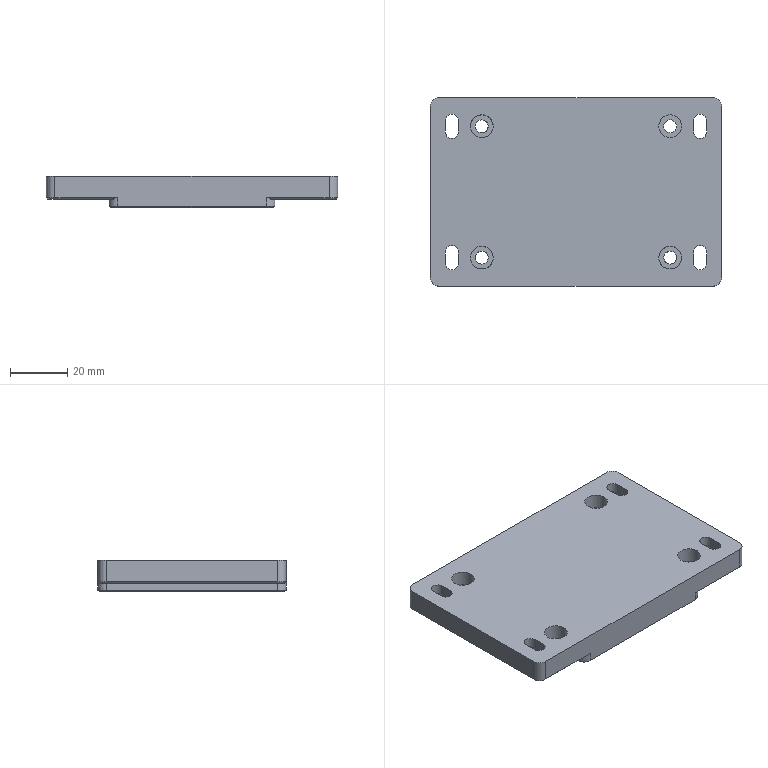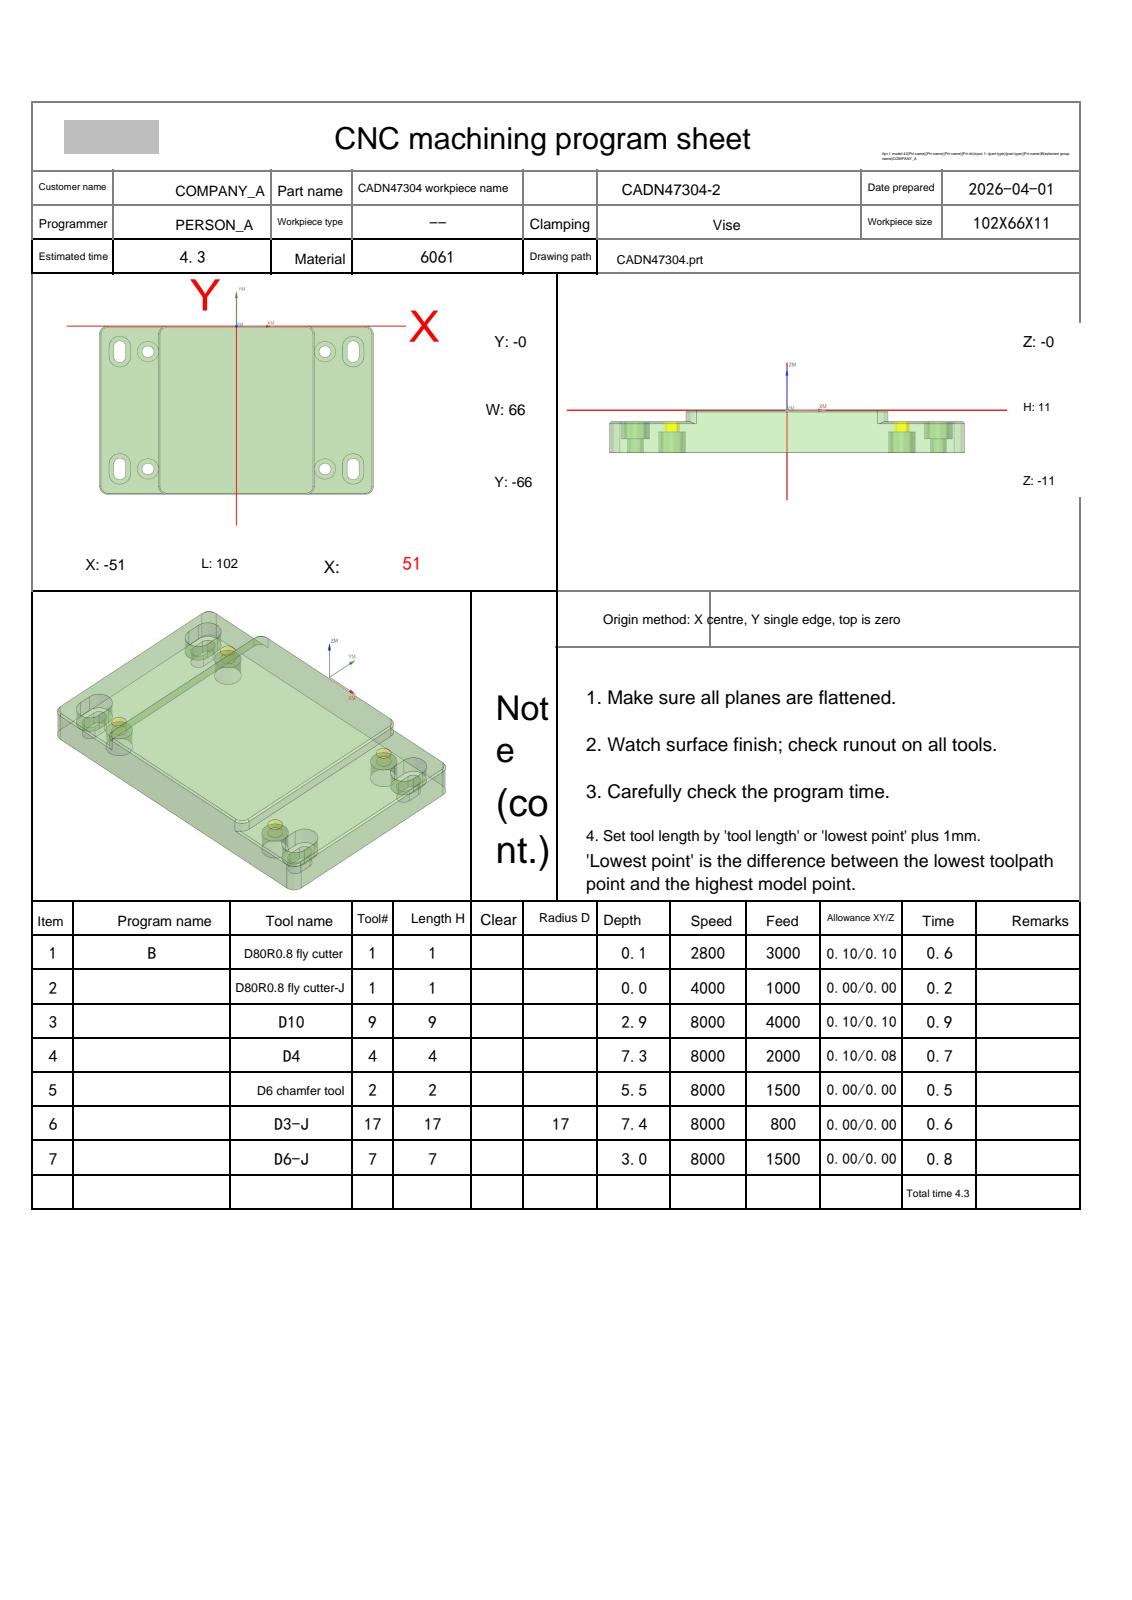NC program | NX | posted by the shop | part box 102 x 66 x 11 mm
Whole program:
%
O0001
(Machine time: 5.73 MIN)
(===Total Tool:6===)
(T1=D80R0.8 fly cutter D=80.  R=0.8  D-  H01 Z=-0.   )
(T9=D10     D=10.  R=0.   D-  H09 Z=-2.9  )
(T4=D4      D=4.   R=0.   D-  H04 Z=-7.34 )
(T2=D6 chamfer tool   D=6.   R=0.   D-  H02 Z=-5.55 )
(T17=D3-J   D=3.   R=0.   D17 H17 Z=-7.4  )
(T7=D6-J    D=6.   R=0.   D7  H07 Z=-3.   )
G80 G90 G17 G49 G40
G91 G28 Z0
M01
N1 T01 M06
(D80R0.8 fly cutter  D=80. R=0.8 H=01 ce=0.10 di=0.10)
G00 G90 G54 X103.097 Y-32.998 M03 S2800
G43 H01 Z20.
M08
Z5.014
G01 Z3.014 F3000.
X91.097
X-91.097 Y-33.002
X-103.097
Z5.014
G00 X103.097 Y-32.998
Z4.529
G01 Z2.529
X91.097
X-91.097 Y-33.002
X-103.097
Z4.529
G00 X103.097 Y-32.998
Z4.043
G01 Z2.043
X91.097
X-91.097 Y-33.002
X-103.097
Z4.043
G00 X103.097 Y-32.998
Z3.557
G01 Z1.557
X91.097
X-91.097 Y-33.002
X-103.097
Z3.557
G00 Z20.
X103.097 Y-32.998
Z3.071
G01 Z1.071
X91.097
X-91.097 Y-33.002
X-103.097
Z3.071
G00 Z20.
X103.097 Y-32.998
Z2.586
G01 Z.586
X91.097
X-91.097 Y-33.002
X-103.097
Z2.586
G00 Z20.
X103.097 Y-32.998
Z2.1
G01 Z.1
X91.097
X-91.097 Y-33.002
X-103.097
Z2.1
G00 Z20.
G91 G28 Z0.0
M05
M09
G91 G28 Z0.0
M01
N2 T01 M06
(D80R0.8 fly cutter-J  D=80. R=0.8 H=01 ce=0.00 di=0.00)
G00 G90 G54 X102.999 Y-32.998 M03 S4000
G43 H01 Z20.
M08
Z2.
G01 Z0.0 F1000.
X90.999
X-90.999 Y-33.002
X-102.999
Z2.
G00 Z20.
G91 G28 Z0.0
M05
M09
G91 G28 Z0.0
M01
N3 T09 M06
(D10  D=10. R=0. H=09 ce=0.10 di=0.10)
G00 G90 G54 X-52.925 Y6.273 M03 S8000
G43 H09 Z13.5
M08
Z.92
G01 Z-.58 F4000.
X-53.701 Y1.718
G03 X-54.1 Y-3. I27.701 J-4.718
G01 Y-63.
G03 X-53.748 Y-67.436 I28.1 J0.0
X-53.504 Y-67.946 I.987 J.158
X-48.778 Y-70.359 I5.504 J4.946
G01 X-48.715 Y-70.362
G03 X-48.115 Y-69.762 I0.0 J.6
G01 X-48.14 Y-69.591
G02 X-49.1 Y-63. I22.14 J6.591
G01 Y-3.
G02 X-48.11 Y3.69 I23.1 J0.0
X-47.153 Y4.4 I.957 J-.29
G01 X-40.704
G02 X-40.104 Y3.8 I0.0 J-.6
X-40.159 Y3.548 I-.6 J0.0
G03 X-41.6 Y-3. I14.159 J-6.548
G01 Y-63.
G03 X-39.963 Y-69.956 I15.6 J0.0
X-39.258 Y-70.492 I.895 J.446
G01 X-29.89 Y-72.296
X-29.701 Y-72.314
G03 X-28.701 Y-71.314 I0.0 J1.
X-29.294 Y-70.4 I-1. J0.0
G02 X-34.1 Y-63. I3.294 J7.4
G01 Y-3.
G02 X-29.294 Y4.4 I8.1 J0.0
G01 X-20.982 Y8.1
Z.92
G00 X-52.925 Y6.273
Z.34
G01 Z-1.16
X-53.701 Y1.718
G03 X-54.1 Y-3. I27.701 J-4.718
G01 Y-63.
G03 X-53.748 Y-67.436 I28.1 J0.0
X-53.504 Y-67.946 I.987 J.158
X-48.778 Y-70.359 I5.504 J4.946
G01 X-48.715 Y-70.362
G03 X-48.115 Y-69.762 I0.0 J.6
G01 X-48.14 Y-69.591
G02 X-49.1 Y-63. I22.14 J6.591
G01 Y-3.
G02 X-48.11 Y3.69 I23.1 J0.0
X-47.153 Y4.4 I.957 J-.29
G01 X-40.704
G02 X-40.104 Y3.8 I0.0 J-.6
X-40.159 Y3.548 I-.6 J0.0
G03 X-41.6 Y-3. I14.159 J-6.548
G01 Y-63.
G03 X-39.963 Y-69.956 I15.6 J0.0
X-39.258 Y-70.492 I.895 J.446
G01 X-29.89 Y-72.296
X-29.701 Y-72.314
G03 X-28.701 Y-71.314 I0.0 J1.
X-29.294 Y-70.4 I-1. J0.0
G02 X-34.1 Y-63. I3.294 J7.4
G01 Y-3.
G02 X-29.294 Y4.4 I8.1 J0.0
G01 X-20.982 Y8.1
Z.34
G00 X-52.925 Y6.273
Z-.24
G01 Z-1.74
X-53.701 Y1.718
G03 X-54.1 Y-3. I27.701 J-4.718
G01 Y-63.
G03 X-53.748 Y-67.436 I28.1 J0.0
X-53.504 Y-67.946 I.987 J.158
X-48.778 Y-70.359 I5.504 J4.946
G01 X-48.715 Y-70.362
G03 X-48.115 Y-69.762 I0.0 J.6
G01 X-48.14 Y-69.591
G02 X-49.1 Y-63. I22.14 J6.591
G01 Y-3.
G02 X-48.11 Y3.69 I23.1 J0.0
X-47.153 Y4.4 I.957 J-.29
G01 X-40.704
G02 X-40.104 Y3.8 I0.0 J-.6
X-40.159 Y3.548 I-.6 J0.0
G03 X-41.6 Y-3. I14.159 J-6.548
G01 Y-63.
G03 X-39.963 Y-69.956 I15.6 J0.0
X-39.258 Y-70.492 I.895 J.446
G01 X-29.89 Y-72.296
X-29.701 Y-72.314
G03 X-28.701 Y-71.314 I0.0 J1.
X-29.294 Y-70.4 I-1. J0.0
G02 X-34.1 Y-63. I3.294 J7.4
G01 Y-3.
G02 X-29.294 Y4.4 I8.1 J0.0
G01 X-20.982 Y8.1
Z-.24
G00 X-52.925 Y6.273
Z-.82
G01 Z-2.32
X-53.701 Y1.718
G03 X-54.1 Y-3. I27.701 J-4.718
G01 Y-63.
G03 X-53.748 Y-67.436 I28.1 J0.0
X-53.504 Y-67.946 I.987 J.158
X-48.778 Y-70.359 I5.504 J4.946
G01 X-48.715 Y-70.362
G03 X-48.115 Y-69.762 I0.0 J.6
G01 X-48.14 Y-69.591
G02 X-49.1 Y-63. I22.14 J6.591
G01 Y-3.
G02 X-48.11 Y3.69 I23.1 J0.0
X-47.153 Y4.4 I.957 J-.29
G01 X-40.704
G02 X-40.104 Y3.8 I0.0 J-.6
X-40.159 Y3.548 I-.6 J0.0
G03 X-41.6 Y-3. I14.159 J-6.548
G01 Y-63.
G03 X-39.963 Y-69.956 I15.6 J0.0
X-39.258 Y-70.492 I.895 J.446
G01 X-29.89 Y-72.296
X-29.701 Y-72.314
G03 X-28.701 Y-71.314 I0.0 J1.
X-29.294 Y-70.4 I-1. J0.0
G02 X-34.1 Y-63. I3.294 J7.4
G01 Y-3.
G02 X-29.294 Y4.4 I8.1 J0.0
G01 X-20.982 Y8.1
Z-.82
G00 X-52.925 Y6.273
Z-1.4
G01 Z-2.9
X-53.701 Y1.718
G03 X-54.1 Y-3. I27.701 J-4.718
G01 Y-63.
G03 X-53.748 Y-67.436 I28.1 J0.0
X-53.504 Y-67.946 I.987 J.158
X-48.778 Y-70.359 I5.504 J4.946
G01 X-48.715 Y-70.362
G03 X-48.115 Y-69.762 I0.0 J.6
G01 X-48.14 Y-69.591
G02 X-49.1 Y-63. I22.14 J6.591
G01 Y-3.
G02 X-48.11 Y3.69 I23.1 J0.0
X-47.153 Y4.4 I.957 J-.29
G01 X-40.704
G02 X-40.104 Y3.8 I0.0 J-.6
X-40.159 Y3.548 I-.6 J0.0
G03 X-41.6 Y-3. I14.159 J-6.548
G01 Y-63.
G03 X-39.963 Y-69.956 I15.6 J0.0
X-39.258 Y-70.492 I.895 J.446
G01 X-29.89 Y-72.296
X-29.701 Y-72.314
G03 X-28.701 Y-71.314 I0.0 J1.
X-29.294 Y-70.4 I-1. J0.0
G02 X-34.1 Y-63. I3.294 J7.4
G01 Y-3.
G02 X-29.294 Y4.4 I8.1 J0.0
G01 X-20.982 Y8.1
Z-1.4
G00 Z13.5
X52.925 Y-72.273
Z.92
G01 Z-.58
X53.701 Y-67.718
G03 X54.1 Y-63. I-27.701 J4.718
G01 Y-3.
G03 X53.748 Y1.436 I-28.1 J0.0
X53.504 Y1.946 I-.987 J-.158
X48.778 Y4.359 I-5.504 J-4.946
G01 X48.715 Y4.362
G03 X48.115 Y3.762 I0.0 J-.6
G01 X48.14 Y3.591
G02 X49.1 Y-3. I-22.14 J-6.591
G01 Y-63.
G02 X48.11 Y-69.69 I-23.1 J0.0
X47.153 Y-70.4 I-.957 J.29
G01 X40.704
G02 X40.104 Y-69.8 I0.0 J.6
X40.159 Y-69.548 I.6 J0.0
G03 X41.6 Y-63. I-14.159 J6.548
G01 Y-3.
G03 X39.963 Y3.956 I-15.6 J0.0
X39.258 Y4.492 I-.895 J-.446
G01 X29.89 Y6.296
X29.701 Y6.314
G03 X28.701 Y5.314 I0.0 J-1.
X29.294 Y4.4 I1. J0.0
G02 X34.1 Y-3. I-3.294 J-7.4
G01 Y-63.
G02 X29.294 Y-70.4 I-8.1 J0.0
G01 X20.982 Y-74.1
Z.92
G00 X52.925 Y-72.273
Z.34
G01 Z-1.16
X53.701 Y-67.718
G03 X54.1 Y-63. I-27.701 J4.718
G01 Y-3.
G03 X53.748 Y1.436 I-28.1 J0.0
X53.504 Y1.946 I-.987 J-.158
X48.778 Y4.359 I-5.504 J-4.946
G01 X48.715 Y4.362
G03 X48.115 Y3.762 I0.0 J-.6
G01 X48.14 Y3.591
G02 X49.1 Y-3. I-22.14 J-6.591
G01 Y-63.
G02 X48.11 Y-69.69 I-23.1 J0.0
X47.153 Y-70.4 I-.957 J.29
G01 X40.704
G02 X40.104 Y-69.8 I0.0 J.6
X40.159 Y-69.548 I.6 J0.0
G03 X41.6 Y-63. I-14.159 J6.548
G01 Y-3.
G03 X39.963 Y3.956 I-15.6 J0.0
X39.258 Y4.492 I-.895 J-.446
G01 X29.89 Y6.296
X29.701 Y6.314
G03 X28.701 Y5.314 I0.0 J-1.
X29.294 Y4.4 I1. J0.0
G02 X34.1 Y-3. I-3.294 J-7.4
G01 Y-63.
G02 X29.294 Y-70.4 I-8.1 J0.0
G01 X20.982 Y-74.1
Z.34
G00 X52.925 Y-72.273
Z-.24
G01 Z-1.74
X53.701 Y-67.718
G03 X54.1 Y-63. I-27.701 J4.718
G01 Y-3.
G03 X53.748 Y1.436 I-28.1 J0.0
X53.504 Y1.946 I-.987 J-.158
X48.778 Y4.359 I-5.504 J-4.946
G01 X48.715 Y4.362
G03 X48.115 Y3.762 I0.0 J-.6
G01 X48.14 Y3.591
G02 X49.1 Y-3. I-22.14 J-6.591
G01 Y-63.
G02 X48.11 Y-69.69 I-23.1 J0.0
X47.153 Y-70.4 I-.957 J.29
G01 X40.704
G02 X40.104 Y-69.8 I0.0 J.6
X40.159 Y-69.548 I.6 J0.0
G03 X41.6 Y-63. I-14.159 J6.548
G01 Y-3.
G03 X39.963 Y3.956 I-15.6 J0.0
X39.258 Y4.492 I-.895 J-.446
G01 X29.89 Y6.296
X29.701 Y6.314
G03 X28.701 Y5.314 I0.0 J-1.
X29.294 Y4.4 I1. J0.0
G02 X34.1 Y-3. I-3.294 J-7.4
G01 Y-63.
G02 X29.294 Y-70.4 I-8.1 J0.0
G01 X20.982 Y-74.1
Z-.24
G00 X52.925 Y-72.273
Z-.82
G01 Z-2.32
X53.701 Y-67.718
G03 X54.1 Y-63. I-27.701 J4.718
G01 Y-3.
G03 X53.748 Y1.436 I-28.1 J0.0
X53.504 Y1.946 I-.987 J-.158
X48.778 Y4.359 I-5.504 J-4.946
G01 X48.715 Y4.362
G03 X48.115 Y3.762 I0.0 J-.6
G01 X48.14 Y3.591
G02 X49.1 Y-3. I-22.14 J-6.591
G01 Y-63.
G02 X48.11 Y-69.69 I-23.1 J0.0
X47.153 Y-70.4 I-.957 J.29
G01 X40.704
G02 X40.104 Y-69.8 I0.0 J.6
X40.159 Y-69.548 I.6 J0.0
G03 X41.6 Y-63. I-14.159 J6.548
G01 Y-3.
G03 X39.963 Y3.956 I-15.6 J0.0
X39.258 Y4.492 I-.895 J-.446
G01 X29.89 Y6.296
X29.701 Y6.314
G03 X28.701 Y5.314 I0.0 J-1.
X29.294 Y4.4 I1. J0.0
G02 X34.1 Y-3. I-3.294 J-7.4
G01 Y-63.
G02 X29.294 Y-70.4 I-8.1 J0.0
G01 X20.982 Y-74.1
Z-.82
G00 X52.925 Y-72.273
Z-1.4
G01 Z-2.9
X53.701 Y-67.718
G03 X54.1 Y-63. I-27.701 J4.718
G01 Y-3.
G03 X53.748 Y1.436 I-28.1 J0.0
X53.504 Y1.946 I-.987 J-.158
X48.778 Y4.359 I-5.504 J-4.946
G01 X48.715 Y4.362
G03 X48.115 Y3.762 I0.0 J-.6
G01 X48.14 Y3.591
G02 X49.1 Y-3. I-22.14 J-6.591
G01 Y-63.
G02 X48.11 Y-69.69 I-23.1 J0.0
X47.153 Y-70.4 I-.957 J.29
G01 X40.704
G02 X40.104 Y-69.8 I0.0 J.6
X40.159 Y-69.548 I.6 J0.0
G03 X41.6 Y-63. I-14.159 J6.548
G01 Y-3.
G03 X39.963 Y3.956 I-15.6 J0.0
X39.258 Y4.492 I-.895 J-.446
G01 X29.89 Y6.296
X29.701 Y6.314
G03 X28.701 Y5.314 I0.0 J-1.
X29.294 Y4.4 I1. J0.0
G02 X34.1 Y-3. I-3.294 J-7.4
G01 Y-63.
G02 X29.294 Y-70.4 I-8.1 J0.0
G01 X20.982 Y-74.1
Z-1.4
G00 Z13.5
G91 G28 Z0.0
M05
M09
G91 G28 Z0.0
M01
N4 T04 M06
(D4  D=4. R=0. H=04 ce=0.10 di=0.08)
G00 G90 G54 X-45.233 Y-12.757 M03 S8000
G43 H04 Z20.
M08
Z-2.2
G01 X-45.112 Y-13.062 Z-2.217 F2000.
X-44.562 Y-13.612 Z-2.258
X-43.839 Y-13.9 Z-2.299
X-43.161 Z-2.334
X-42.438 Y-13.612 Z-2.375
X-41.888 Y-13.062 Z-2.416
X-41.6 Y-12.339 Z-2.457
Y-7.661 Z-2.702
X-41.839 Y-7.017 Z-2.738
X-42.282 Y-6.503 Z-2.773
X-42.696 Y-6.246 Z-2.799
X-43.161 Y-6.1 Z-2.824
X-43.839 Z-2.86
X-44.562 Y-6.388 Z-2.901
X-45.112 Y-6.938 Z-2.941
X-45.4 Y-7.661 Z-2.982
Y-8. Z-3.
Y-12. Z-3.058
G03 X-43.5 Y-13.9 Z-3.101 I1.9 J0.0
X-41.6 Y-12. Z-3.145 I0.0 J1.9
G01 Y-8. Z-3.203
G03 X-42.061 Y-6.76 Z-3.222 I-1.9 J0.0
X-43.5 Y-6.1 Z-3.246 I-1.439 J-1.24
X-45.4 Y-8. Z-3.289 I0.0 J-1.9
G01 Y-12. Z-3.347
G03 X-43.5 Y-13.9 Z-3.391 I1.9 J0.0
X-41.6 Y-12. Z-3.434 I0.0 J1.9
G01 Y-8. Z-3.492
G03 X-42.061 Y-6.76 Z-3.512 I-1.9 J0.0
X-43.5 Y-6.1 Z-3.535 I-1.439 J-1.24
X-45.4 Y-8. Z-3.579 I0.0 J-1.9
G01 Y-12. Z-3.637
G03 X-43.5 Y-13.9 Z-3.68 I1.9 J0.0
X-41.6 Y-12. Z-3.723 I0.0 J1.9
G01 Y-8. Z-3.781
G03 X-42.061 Y-6.76 Z-3.801 I-1.9 J0.0
X-43.5 Y-6.1 Z-3.825 I-1.439 J-1.24
X-45.4 Y-8. Z-3.868 I0.0 J-1.9
G01 Y-12. Z-3.926
G03 X-43.5 Y-13.9 Z-3.969 I1.9 J0.0
X-41.6 Y-12. Z-4.013 I0.0 J1.9
G01 Y-8. Z-4.071
G03 X-42.061 Y-6.76 Z-4.09 I-1.9 J0.0
X-43.5 Y-6.1 Z-4.114 I-1.439 J-1.24
X-45.4 Y-8. Z-4.157 I0.0 J-1.9
G01 Y-12. Z-4.215
G03 X-43.5 Y-13.9 Z-4.259 I1.9 J0.0
X-41.6 Y-12. Z-4.302 I0.0 J1.9
G01 Y-8. Z-4.36
G03 X-42.061 Y-6.76 Z-4.38 I-1.9 J0.0
X-43.5 Y-6.1 Z-4.403 I-1.439 J-1.24
X-45.4 Y-8. Z-4.447 I0.0 J-1.9
G01 Y-12. Z-4.505
G03 X-43.5 Y-13.9 Z-4.548 I1.9 J0.0
X-41.6 Y-12. Z-4.591 I0.0 J1.9
G01 Y-8. Z-4.649
G03 X-42.061 Y-6.76 Z-4.669 I-1.9 J0.0
X-43.5 Y-6.1 Z-4.693 I-1.439 J-1.24
X-45.4 Y-8. Z-4.736 I0.0 J-1.9
G01 Y-12. Z-4.794
G03 X-43.5 Y-13.9 Z-4.837 I1.9 J0.0
X-41.6 Y-12. Z-4.881 I0.0 J1.9
G01 Y-8. Z-4.939
G03 X-42.061 Y-6.76 Z-4.958 I-1.9 J0.0
X-43.5 Y-6.1 Z-4.982 I-1.439 J-1.24
X-45.4 Y-8. Z-5.025 I0.0 J-1.9
G01 Y-12. Z-5.083
G03 X-43.5 Y-13.9 Z-5.127 I1.9 J0.0
X-41.6 Y-12. Z-5.17 I0.0 J1.9
G01 Y-8. Z-5.228
G03 X-42.061 Y-6.76 Z-5.248 I-1.9 J0.0
X-43.5 Y-6.1 Z-5.271 I-1.439 J-1.24
X-45.4 Y-8. Z-5.315 I0.0 J-1.9
G01 Y-12. Z-5.373
G03 X-43.5 Y-13.9 Z-5.416 I1.9 J0.0
X-41.6 Y-12. Z-5.459 I0.0 J1.9
G01 Y-8. Z-5.517
G03 X-42.061 Y-6.76 Z-5.537 I-1.9 J0.0
X-43.5 Y-6.1 Z-5.561 I-1.439 J-1.24
X-45.4 Y-8. Z-5.604 I0.0 J-1.9
G01 Y-12. Z-5.662
G03 X-43.5 Y-13.9 Z-5.705 I1.9 J0.0
X-41.6 Y-12. Z-5.749 I0.0 J1.9
G01 Y-8. Z-5.807
G03 X-42.061 Y-6.76 Z-5.826 I-1.9 J0.0
X-43.5 Y-6.1 Z-5.85 I-1.439 J-1.24
X-45.4 Y-8. Z-5.893 I0.0 J-1.9
G01 Y-12. Z-5.951
G03 X-43.5 Y-13.9 Z-5.995 I1.9 J0.0
X-41.6 Y-12. Z-6.038 I0.0 J1.9
G01 Y-8. Z-6.096
G03 X-42.061 Y-6.76 Z-6.116 I-1.9 J0.0
X-43.5 Y-6.1 Z-6.139 I-1.439 J-1.24
X-45.4 Y-8. Z-6.183 I0.0 J-1.9
G01 Y-12. Z-6.241
G03 X-43.5 Y-13.9 Z-6.284 I1.9 J0.0
X-41.6 Y-12. Z-6.327 I0.0 J1.9
G01 Y-8. Z-6.385
G03 X-42.061 Y-6.76 Z-6.405 I-1.9 J0.0
X-43.5 Y-6.1 Z-6.429 I-1.439 J-1.24
X-45.4 Y-8. Z-6.472 I0.0 J-1.9
G01 Y-12. Z-6.53
G03 X-43.5 Y-13.9 Z-6.573 I1.9 J0.0
X-41.6 Y-12. Z-6.617 I0.0 J1.9
G01 Y-8. Z-6.675
G03 X-42.061 Y-6.76 Z-6.694 I-1.9 J0.0
X-43.5 Y-6.1 Z-6.718 I-1.439 J-1.24
X-45.4 Y-8. Z-6.761 I0.0 J-1.9
G01 Y-12. Z-6.819
G03 X-43.5 Y-13.9 Z-6.863 I1.9 J0.0
X-41.6 Y-12. Z-6.906 I0.0 J1.9
G01 Y-8. Z-6.964
G03 X-42.061 Y-6.76 Z-6.984 I-1.9 J0.0
X-43.5 Y-6.1 Z-7.007 I-1.439 J-1.24
X-45.4 Y-8. Z-7.051 I0.0 J-1.9
G01 Y-12. Z-7.109
G03 X-43.5 Y-13.9 Z-7.152 I1.9 J0.0
X-41.6 Y-12. Z-7.195 I0.0 J1.9
G01 Y-8. Z-7.253
G03 X-42.061 Y-6.76 Z-7.273 I-1.9 J0.0
X-43.5 Y-6.1 Z-7.297 I-1.439 J-1.24
X-45.4 Y-8. Z-7.34 I0.0 J-1.9
G01 Y-12.
G03 X-43.5 Y-13.9 I1.9 J0.0
X-41.6 Y-12. I0.0 J1.9
G01 Y-8.
G03 X-43.5 Y-6.1 I-1.9 J0.0
X-45.4 Y-8. I0.0 J-1.9
G01 Y-8.4
Z-6.54
G00 Z20.
X-45.235 Y-58.752
Z-2.2
G01 X-45.112 Y-59.062 Z-2.217
X-44.562 Y-59.612 Z-2.258
X-43.839 Y-59.9 Z-2.299
X-43.161 Z-2.335
X-42.438 Y-59.612 Z-2.375
X-41.888 Y-59.062 Z-2.416
X-41.6 Y-58.339 Z-2.457
Y-53.661 Z-2.702
X-41.888 Y-52.938 Z-2.743
X-42.438 Y-52.388 Z-2.784
X-43.161 Y-52.1 Z-2.824
X-43.839 Z-2.86
X-44.562 Y-52.388 Z-2.901
X-45.112 Y-52.938 Z-2.941
X-45.4 Y-53.661 Z-2.982
Y-54. Z-3.
Y-58. Z-3.058
G03 X-43.5 Y-59.9 Z-3.101 I1.9 J0.0
X-41.6 Y-58. Z-3.145 I0.0 J1.9
G01 Y-54. Z-3.203
G03 X-43.5 Y-52.1 Z-3.246 I-1.9 J0.0
X-45.4 Y-54. Z-3.289 I0.0 J-1.9
G01 Y-58. Z-3.347
G03 X-43.5 Y-59.9 Z-3.391 I1.9 J0.0
X-41.6 Y-58. Z-3.434 I0.0 J1.9
G01 Y-54. Z-3.492
G03 X-43.5 Y-52.1 Z-3.535 I-1.9 J0.0
X-45.4 Y-54. Z-3.579 I0.0 J-1.9
G01 Y-58. Z-3.637
G03 X-43.5 Y-59.9 Z-3.68 I1.9 J0.0
X-41.6 Y-58. Z-3.723 I0.0 J1.9
G01 Y-54. Z-3.781
G03 X-43.5 Y-52.1 Z-3.825 I-1.9 J0.0
X-45.4 Y-54. Z-3.868 I0.0 J-1.9
G01 Y-58. Z-3.926
G03 X-43.5 Y-59.9 Z-3.969 I1.9 J0.0
X-41.6 Y-58. Z-4.013 I0.0 J1.9
G01 Y-54. Z-4.071
G03 X-43.5 Y-52.1 Z-4.114 I-1.9 J0.0
X-45.4 Y-54. Z-4.157 I0.0 J-1.9
G01 Y-58. Z-4.215
G03 X-43.5 Y-59.9 Z-4.259 I1.9 J0.0
X-41.6 Y-58. Z-4.302 I0.0 J1.9
G01 Y-54. Z-4.36
G03 X-43.5 Y-52.1 Z-4.403 I-1.9 J0.0
X-45.4 Y-54. Z-4.447 I0.0 J-1.9
G01 Y-58. Z-4.505
G03 X-43.5 Y-59.9 Z-4.548 I1.9 J0.0
X-41.6 Y-58. Z-4.591 I0.0 J1.9
G01 Y-54. Z-4.649
G03 X-43.5 Y-52.1 Z-4.693 I-1.9 J0.0
X-45.4 Y-54. Z-4.736 I0.0 J-1.9
G01 Y-58. Z-4.794
G03 X-43.5 Y-59.9 Z-4.837 I1.9 J0.0
X-41.6 Y-58. Z-4.881 I0.0 J1.9
G01 Y-54. Z-4.939
G03 X-43.5 Y-52.1 Z-4.982 I-1.9 J0.0
X-45.4 Y-54. Z-5.025 I0.0 J-1.9
G01 Y-58. Z-5.083
G03 X-43.5 Y-59.9 Z-5.127 I1.9 J0.0
X-41.6 Y-58. Z-5.17 I0.0 J1.9
G01 Y-54. Z-5.228
G03 X-43.5 Y-52.1 Z-5.271 I-1.9 J0.0
X-45.4 Y-54. Z-5.315 I0.0 J-1.9
G01 Y-58. Z-5.373
G03 X-43.5 Y-59.9 Z-5.416 I1.9 J0.0
X-41.6 Y-58. Z-5.459 I0.0 J1.9
G01 Y-54. Z-5.517
G03 X-43.5 Y-52.1 Z-5.561 I-1.9 J0.0
X-45.4 Y-54. Z-5.604 I0.0 J-1.9
G01 Y-58. Z-5.662
G03 X-43.5 Y-59.9 Z-5.705 I1.9 J0.0
X-41.6 Y-58. Z-5.749 I0.0 J1.9
G01 Y-54. Z-5.807
G03 X-43.5 Y-52.1 Z-5.85 I-1.9 J0.0
X-45.4 Y-54. Z-5.893 I0.0 J-1.9
G01 Y-58. Z-5.951
G03 X-43.5 Y-59.9 Z-5.995 I1.9 J0.0
X-41.6 Y-58. Z-6.038 I0.0 J1.9
G01 Y-54. Z-6.096
G03 X-43.5 Y-52.1 Z-6.139 I-1.9 J0.0
X-45.4 Y-54. Z-6.183 I0.0 J-1.9
G01 Y-58. Z-6.241
G03 X-43.5 Y-59.9 Z-6.284 I1.9 J0.0
X-41.6 Y-58. Z-6.327 I0.0 J1.9
G01 Y-54. Z-6.385
G03 X-43.5 Y-52.1 Z-6.429 I-1.9 J0.0
X-45.4 Y-54. Z-6.472 I0.0 J-1.9
G01 Y-58. Z-6.53
G03 X-43.5 Y-59.9 Z-6.573 I1.9 J0.0
X-41.6 Y-58. Z-6.617 I0.0 J1.9
G01 Y-54. Z-6.675
G03 X-43.5 Y-52.1 Z-6.718 I-1.9 J0.0
X-45.4 Y-54. Z-6.761 I0.0 J-1.9
G01 Y-58. Z-6.819
G03 X-43.5 Y-59.9 Z-6.863 I1.9 J0.0
X-41.6 Y-58. Z-6.906 I0.0 J1.9
G01 Y-54. Z-6.964
G03 X-43.5 Y-52.1 Z-7.007 I-1.9 J0.0
X-45.4 Y-54. Z-7.051 I0.0 J-1.9
G01 Y-58. Z-7.109
G03 X-43.5 Y-59.9 Z-7.152 I1.9 J0.0
X-41.6 Y-58. Z-7.195 I0.0 J1.9
G01 Y-54. Z-7.253
G03 X-43.5 Y-52.1 Z-7.297 I-1.9 J0.0
X-45.4 Y-54. Z-7.34 I0.0 J-1.9
G01 Y-58.
G03 X-43.5 Y-59.9 I1.9 J0.0
X-41.6 Y-58. I0.0 J1.9
G01 Y-54.
G03 X-43.5 Y-52.1 I-1.9 J0.0
X-45.4 Y-54. I0.0 J-1.9
G01 Y-54.4
Z-6.54
G00 Z20.
X45.235 Y-53.249
Z-2.2
G01 X45.112 Y-52.938 Z-2.217
X44.562 Y-52.388 Z-2.258
X43.839 Y-52.1 Z-2.299
X43.161 Z-2.335
X42.438 Y-52.388 Z-2.375
X41.888 Y-52.938 Z-2.416
X41.6 Y-53.661 Z-2.457
Y-58.339 Z-2.702
X41.888 Y-59.062 Z-2.743
X42.438 Y-59.612 Z-2.784
X43.161 Y-59.9 Z-2.824
X43.839 Z-2.86
X44.562 Y-59.612 Z-2.901
X45.112 Y-59.062 Z-2.941
X45.4 Y-58.339 Z-2.982
Y-58. Z-3.
Y-54. Z-3.058
G03 X43.5 Y-52.1 Z-3.101 I-1.9 J0.0
X41.6 Y-54. Z-3.145 I0.0 J-1.9
G01 Y-58. Z-3.203
G03 X43.5 Y-59.9 Z-3.246 I1.9 J0.0
X45.4 Y-58. Z-3.289 I0.0 J1.9
G01 Y-54. Z-3.347
G03 X43.5 Y-52.1 Z-3.391 I-1.9 J0.0
X41.6 Y-54. Z-3.434 I0.0 J-1.9
G01 Y-58. Z-3.492
G03 X43.5 Y-59.9 Z-3.535 I1.9 J0.0
X45.4 Y-58. Z-3.579 I0.0 J1.9
G01 Y-54. Z-3.637
G03 X43.5 Y-52.1 Z-3.68 I-1.9 J0.0
X41.6 Y-54. Z-3.723 I0.0 J-1.9
G01 Y-58. Z-3.781
G03 X43.5 Y-59.9 Z-3.825 I1.9 J0.0
X45.4 Y-58. Z-3.868 I0.0 J1.9
G01 Y-54. Z-3.926
G03 X43.5 Y-52.1 Z-3.969 I-1.9 J0.0
X41.6 Y-54. Z-4.013 I0.0 J-1.9
G01 Y-58. Z-4.071
G03 X43.5 Y-59.9 Z-4.114 I1.9 J0.0
X45.4 Y-58. Z-4.157 I0.0 J1.9
G01 Y-54. Z-4.215
G03 X43.5 Y-52.1 Z-4.259 I-1.9 J0.0
X41.6 Y-54. Z-4.302 I0.0 J-1.9
G01 Y-58. Z-4.36
G03 X43.5 Y-59.9 Z-4.403 I1.9 J0.0
X45.4 Y-58. Z-4.447 I0.0 J1.9
G01 Y-54. Z-4.505
G03 X43.5 Y-52.1 Z-4.548 I-1.9 J0.0
X41.6 Y-54. Z-4.591 I0.0 J-1.9
G01 Y-58. Z-4.649
G03 X43.5 Y-59.9 Z-4.693 I1.9 J0.0
X45.4 Y-58. Z-4.736 I0.0 J1.9
G01 Y-54. Z-4.794
G03 X43.5 Y-52.1 Z-4.837 I-1.9 J0.0
X41.6 Y-54. Z-4.881 I0.0 J-1.9
G01 Y-58. Z-4.939
G03 X43.5 Y-59.9 Z-4.982 I1.9 J0.0
X45.4 Y-58. Z-5.025 I0.0 J1.9
G01 Y-54. Z-5.083
G03 X43.5 Y-52.1 Z-5.127 I-1.9 J0.0
X41.6 Y-54. Z-5.17 I0.0 J-1.9
G01 Y-58. Z-5.228
G03 X43.5 Y-59.9 Z-5.271 I1.9 J0.0
X45.4 Y-58. Z-5.315 I0.0 J1.9
G01 Y-54. Z-5.373
G03 X43.5 Y-52.1 Z-5.416 I-1.9 J0.0
X41.6 Y-54. Z-5.459 I0.0 J-1.9
G01 Y-58. Z-5.517
G03 X43.5 Y-59.9 Z-5.561 I1.9 J0.0
X45.4 Y-58. Z-5.604 I0.0 J1.9
G01 Y-54. Z-5.662
G03 X43.5 Y-52.1 Z-5.705 I-1.9 J0.0
X41.6 Y-54. Z-5.749 I0.0 J-1.9
G01 Y-58. Z-5.807
G03 X43.5 Y-59.9 Z-5.85 I1.9 J0.0
X45.4 Y-58. Z-5.893 I0.0 J1.9
G01 Y-54. Z-5.951
G03 X43.5 Y-52.1 Z-5.995 I-1.9 J0.0
X41.6 Y-54. Z-6.038 I0.0 J-1.9
G01 Y-58. Z-6.096
G03 X43.5 Y-59.9 Z-6.139 I1.9 J0.0
X45.4 Y-58. Z-6.183 I0.0 J1.9
G01 Y-54. Z-6.241
G03 X43.5 Y-52.1 Z-6.284 I-1.9 J0.0
X41.6 Y-54. Z-6.327 I0.0 J-1.9
G01 Y-58. Z-6.385
G03 X43.5 Y-59.9 Z-6.429 I1.9 J0.0
X45.4 Y-58. Z-6.472 I0.0 J1.9
G01 Y-54. Z-6.53
G03 X43.5 Y-52.1 Z-6.573 I-1.9 J0.0
X41.6 Y-54. Z-6.617 I0.0 J-1.9
G01 Y-58. Z-6.675
G03 X43.5 Y-59.9 Z-6.718 I1.9 J0.0
X45.4 Y-58. Z-6.761 I0.0 J1.9
G01 Y-54. Z-6.819
G03 X43.5 Y-52.1 Z-6.863 I-1.9 J0.0
X41.6 Y-54. Z-6.906 I0.0 J-1.9
G01 Y-58. Z-6.964
G03 X43.5 Y-59.9 Z-7.007 I1.9 J0.0
X45.4 Y-58. Z-7.051 I0.0 J1.9
G01 Y-54. Z-7.109
G03 X43.5 Y-52.1 Z-7.152 I-1.9 J0.0
X41.6 Y-54. Z-7.195 I0.0 J-1.9
G01 Y-58. Z-7.253
G03 X43.5 Y-59.9 Z-7.297 I1.9 J0.0
X45.4 Y-58. Z-7.34 I0.0 J1.9
G01 Y-54.
G03 X43.5 Y-52.1 I-1.9 J0.0
X41.6 Y-54. I0.0 J-1.9
G01 Y-58.
G03 X43.5 Y-59.9 I1.9 J0.0
X45.4 Y-58. I0.0 J1.9
G01 Y-57.6
Z-6.54
G00 Z20.
X45.235 Y-7.249
Z-2.2
G01 X45.112 Y-6.938 Z-2.217
X44.562 Y-6.388 Z-2.258
X43.839 Y-6.1 Z-2.299
X43.161 Z-2.335
X42.438 Y-6.388 Z-2.375
X41.888 Y-6.938 Z-2.416
X41.6 Y-7.661 Z-2.457
Y-12.339 Z-2.702
X41.888 Y-13.062 Z-2.743
X42.438 Y-13.612 Z-2.784
X43.161 Y-13.9 Z-2.824
X43.839 Z-2.86
X44.562 Y-13.612 Z-2.901
X45.112 Y-13.062 Z-2.941
X45.4 Y-12.339 Z-2.982
Y-12. Z-3.
Y-8. Z-3.058
G03 X43.5 Y-6.1 Z-3.101 I-1.9 J0.0
X41.6 Y-8. Z-3.145 I0.0 J-1.9
G01 Y-12. Z-3.203
G03 X43.5 Y-13.9 Z-3.246 I1.9 J0.0
X45.4 Y-12. Z-3.289 I0.0 J1.9
G01 Y-8. Z-3.347
G03 X43.5 Y-6.1 Z-3.391 I-1.9 J0.0
X41.6 Y-8. Z-3.434 I0.0 J-1.9
G01 Y-12. Z-3.492
G03 X43.5 Y-13.9 Z-3.535 I1.9 J0.0
X45.4 Y-12. Z-3.579 I0.0 J1.9
G01 Y-8. Z-3.637
G03 X43.5 Y-6.1 Z-3.68 I-1.9 J0.0
X41.6 Y-8. Z-3.723 I0.0 J-1.9
G01 Y-12. Z-3.781
G03 X43.5 Y-13.9 Z-3.825 I1.9 J0.0
X45.4 Y-12. Z-3.868 I0.0 J1.9
G01 Y-8. Z-3.926
G03 X43.5 Y-6.1 Z-3.969 I-1.9 J0.0
X41.6 Y-8. Z-4.013 I0.0 J-1.9
G01 Y-12. Z-4.071
G03 X43.5 Y-13.9 Z-4.114 I1.9 J0.0
X45.4 Y-12. Z-4.157 I0.0 J1.9
G01 Y-8. Z-4.215
G03 X43.5 Y-6.1 Z-4.259 I-1.9 J0.0
X41.6 Y-8. Z-4.302 I0.0 J-1.9
G01 Y-12. Z-4.36
G03 X43.5 Y-13.9 Z-4.403 I1.9 J0.0
X45.4 Y-12. Z-4.447 I0.0 J1.9
G01 Y-8. Z-4.505
G03 X43.5 Y-6.1 Z-4.548 I-1.9 J0.0
X41.6 Y-8. Z-4.591 I0.0 J-1.9
G01 Y-12. Z-4.649
G03 X43.5 Y-13.9 Z-4.693 I1.9 J0.0
X45.4 Y-12. Z-4.736 I0.0 J1.9
G01 Y-8. Z-4.794
G03 X43.5 Y-6.1 Z-4.837 I-1.9 J0.0
X41.6 Y-8. Z-4.881 I0.0 J-1.9
G01 Y-12. Z-4.939
G03 X43.5 Y-13.9 Z-4.982 I1.9 J0.0
X45.4 Y-12. Z-5.025 I0.0 J1.9
G01 Y-8. Z-5.083
G03 X43.5 Y-6.1 Z-5.127 I-1.9 J0.0
X41.6 Y-8. Z-5.17 I0.0 J-1.9
G01 Y-12. Z-5.228
G03 X43.5 Y-13.9 Z-5.271 I1.9 J0.0
X45.4 Y-12. Z-5.315 I0.0 J1.9
G01 Y-8. Z-5.373
G03 X43.5 Y-6.1 Z-5.416 I-1.9 J0.0
X41.6 Y-8. Z-5.459 I0.0 J-1.9
G01 Y-12. Z-5.517
G03 X43.5 Y-13.9 Z-5.561 I1.9 J0.0
X45.4 Y-12. Z-5.604 I0.0 J1.9
G01 Y-8. Z-5.662
G03 X43.5 Y-6.1 Z-5.705 I-1.9 J0.0
X41.6 Y-8. Z-5.749 I0.0 J-1.9
G01 Y-12. Z-5.807
G03 X43.5 Y-13.9 Z-5.85 I1.9 J0.0
X45.4 Y-12. Z-5.893 I0.0 J1.9
G01 Y-8. Z-5.951
G03 X43.5 Y-6.1 Z-5.995 I-1.9 J0.0
X41.6 Y-8. Z-6.038 I0.0 J-1.9
G01 Y-12. Z-6.096
G03 X43.5 Y-13.9 Z-6.139 I1.9 J0.0
X45.4 Y-12. Z-6.183 I0.0 J1.9
G01 Y-8. Z-6.241
G03 X43.5 Y-6.1 Z-6.284 I-1.9 J0.0
X41.6 Y-8. Z-6.327 I0.0 J-1.9
G01 Y-12. Z-6.385
G03 X43.5 Y-13.9 Z-6.429 I1.9 J0.0
X45.4 Y-12. Z-6.472 I0.0 J1.9
G01 Y-8. Z-6.53
G03 X43.5 Y-6.1 Z-6.573 I-1.9 J0.0
X41.6 Y-8. Z-6.617 I0.0 J-1.9
G01 Y-12. Z-6.675
G03 X43.5 Y-13.9 Z-6.718 I1.9 J0.0
X45.4 Y-12. Z-6.761 I0.0 J1.9
G01 Y-8. Z-6.819
G03 X43.5 Y-6.1 Z-6.863 I-1.9 J0.0
X41.6 Y-8. Z-6.906 I0.0 J-1.9
G01 Y-12. Z-6.964
G03 X43.5 Y-13.9 Z-7.007 I1.9 J0.0
X45.4 Y-12. Z-7.051 I0.0 J1.9
G01 Y-8. Z-7.109
G03 X43.5 Y-6.1 Z-7.152 I-1.9 J0.0
X41.6 Y-8. Z-7.195 I0.0 J-1.9
G01 Y-12. Z-7.253
G03 X43.5 Y-13.9 Z-7.297 I1.9 J0.0
X45.4 Y-12. Z-7.34 I0.0 J1.9
G01 Y-8.
G03 X43.5 Y-6.1 I-1.9 J0.0
X41.6 Y-8. I0.0 J-1.9
G01 Y-12.
G03 X43.5 Y-13.9 I1.9 J0.0
X45.4 Y-12. I0.0 J1.9
G01 Y-11.6
Z-6.54
G00 Z20.
G91 G28 Z0.0
M05
M09
G91 G28 Z0.0
M01
N5 T02 M06
(D6 chamfer tool  D=6. R=0. H=02 ce=0.00 di=0.08)
G00 G90 G54 X33. Y-10. M03 S8000
G43 H02 Z20.
M08
G98 G81 X33. Y-10. Z-5.55 R0.0 F1000.
Y-56.
X-33.
Y-10.
G80
G00 Z20.
G00 G90 X32.197 Y-56.865 M03 S6500
Z20.
Z-2.127
G01 Z-4.199 F1500.
X32.214 Y-56.934
X32.256 Y-56.992
X32.261 Y-57.015
X32.285 Y-57.021
G03 X33.004 Y-57.249 I.719 J1.017
X34.223 Y-56.26 I0.0 J1.246
X34.25 Y-56. I-1.223 J.26
X33. Y-54.75 I-1.25 J0.0
X32.783 Y-54.769 I0.0 J-1.25
G01 X32.505 Y-54.852
X32.285 Y-54.979
X32.261 Y-54.985
X32.256 Y-55.008
X32.214 Y-55.066
X32.197 Y-55.135
Z-2.127
G00 Z-.449
X40.727 Y-55.614
Z-2.828
G01 Z-4.199
G03 X40.527 Y-55.9 I1.532 J-1.286
G01 X40.497 Y-55.946
X40.5 Y-56.
Y-58.
G03 X43.5 Y-61. I3. J0.0
X46.5 Y-58. I0.0 J3.
G01 Y-54.
G03 X43.5 Y-51. I-3. J0.0
X40.5 Y-54. I0.0 J-3.
G01 Y-56.
X40.497 Y-56.054
X40.527 Y-56.1
G03 X40.727 Y-56.386 I1.732 J1.
G01 Z-2.828
G00 Z10.
Y-9.614
Z-2.828
G01 Z-4.199
G03 X40.527 Y-9.9 I1.532 J-1.286
G01 X40.497 Y-9.946
X40.5 Y-10.
Y-12.
G03 X43.5 Y-15. I3. J0.0
X46.5 Y-12. I0.0 J3.
G01 Y-8.
G03 X43.5 Y-5. I-3. J0.0
X40.5 Y-8. I0.0 J-3.
G01 Y-10.
X40.497 Y-10.054
X40.527 Y-10.1
G03 X40.727 Y-10.386 I1.732 J1.
G01 Z-2.828
G00 Z-.449
X32.197 Y-10.865
Z-2.127
G01 Z-4.199
X32.214 Y-10.934
X32.256 Y-10.992
X32.261 Y-11.015
X32.285 Y-11.021
G03 X33.004 Y-11.249 I.719 J1.017
X34.223 Y-10.26 I0.0 J1.246
X34.25 Y-10. I-1.223 J.26
X33. Y-8.75 I-1.25 J0.0
X32.783 Y-8.769 I0.0 J-1.25
G01 X32.505 Y-8.852
X32.285 Y-8.979
X32.261 Y-8.985
X32.256 Y-9.008
X32.214 Y-9.066
X32.197 Y-9.135
Z-2.127
G00 Z10.
X-32.206 Y-9.18
Z-2.127
G01 Z-4.199
X-32.222 Y-9.093
X-32.263 Y-9.015
X-32.269 Y-8.987
X-32.296 Y-8.975
X-32.375 Y-8.917
G03 X-33. Y-8.75 I-.625 J-1.083
X-34.25 Y-10. I0.0 J-1.25
X-33. Y-11.25 I1.25 J0.0
X-32.375 Y-11.083 I0.0 J1.25
G01 X-32.296 Y-11.025
X-32.277 Y-11.007
X-32.248 Y-10.988
X-32.244 Y-10.954
G03 X-32.202 Y-10.749 I-1.15 J.343
G01 Z-2.127
G00 Z10.
X-46.273 Y-9.614
Z-2.828
G01 Z-4.199
G03 X-46.473 Y-9.9 I1.532 J-1.286
G01 X-46.503 Y-9.946
X-46.5 Y-10.
Y-12.
G03 X-43.5 Y-15. I3. J0.0
X-40.5 Y-12. I0.0 J3.
G01 Y-8.
G03 X-43.5 Y-5. I-3. J0.0
X-46.5 Y-8. I0.0 J-3.
G01 Y-10.
X-46.503 Y-10.054
X-46.473 Y-10.1
G03 X-46.273 Y-10.386 I1.732 J1.
G01 Z-2.828
G00 Z10.
Y-55.614
Z-2.828
G01 Z-4.199
G03 X-46.473 Y-55.9 I1.532 J-1.286
G01 X-46.503 Y-55.946
X-46.5 Y-56.
Y-58.
G03 X-43.5 Y-61. I3. J0.0
X-40.5 Y-58. I0.0 J3.
G01 Y-54.
G03 X-43.5 Y-51. I-3. J0.0
X-46.5 Y-54. I0.0 J-3.
G01 Y-56.
X-46.503 Y-56.054
X-46.473 Y-56.1
G03 X-46.273 Y-56.386 I1.732 J1.
G01 Z-2.828
G00 Z10.
X-32.206 Y-55.18
Z-2.127
G01 Z-4.199
X-32.222 Y-55.093
X-32.263 Y-55.015
X-32.269 Y-54.987
X-32.296 Y-54.975
X-32.375 Y-54.917
G03 X-33. Y-54.75 I-.625 J-1.083
X-34.25 Y-56. I0.0 J-1.25
X-33. Y-57.25 I1.25 J0.0
X-32.375 Y-57.083 I0.0 J1.25
G01 X-32.296 Y-57.025
X-32.277 Y-57.007
X-32.248 Y-56.988
X-32.244 Y-56.954
G03 X-32.202 Y-56.749 I-1.15 J.343
G01 Z-2.127
G00 Z20.
G00 G90 X30.727 Y-32.614 M03 S6500
Z20.
Z-.828
G01 Z-1.999 F1500.
G03 X30.527 Y-32.9 I1.532 J-1.286
G01 X30.497 Y-32.946
X30.5 Y-33.
Y-63.
G02 X26. Y-67.5 I-4.5 J0.0
G01 X-26.
G02 X-30.5 Y-63. I0.0 J4.5
G01 Y-3.
G02 X-26. Y1.5 I4.5 J0.0
G01 X26.
G02 X30.5 Y-3. I0.0 J-4.5
G01 Y-33.
X30.497 Y-33.054
X30.527 Y-33.1
G03 X30.727 Y-33.386 I1.732 J1.
G01 Z-.828
G00 Z10.
X30.014 Y1.727
Z-2.127
G01 Z-4.999
G03 X30.3 Y1.527 I1.286 J1.532
G01 X30.345 Y1.497
X30.4 Y1.5
X48.
G02 X52.5 Y-3. I0.0 J-4.5
G01 Y-63.
G02 X48. Y-67.5 I-4.5 J0.0
G01 X30.4
X30.345 Y-67.497
X30.3 Y-67.527
G03 X30.014 Y-67.727 I1. J-1.732
G01 Z-2.127
G00 Z10.
X-30.014
Z-2.127
G01 Z-4.999
G03 X-30.3 Y-67.527 I-1.286 J-1.532
G01 X-30.345 Y-67.497
X-30.4 Y-67.5
X-48.
G02 X-52.5 Y-63. I0.0 J4.5
G01 Y-3.
G02 X-48. Y1.5 I4.5 J0.0
G01 X-30.4
X-30.345 Y1.497
X-30.3 Y1.527
G03 X-30.014 Y1.727 I-1. J1.732
G01 Z-2.127
G00 Z20.
G91 G28 Z0.0
M05
M09
G91 G28 Z0.0
M01
N6 T17 M06
(D3-J  D=3. R=0. H=17 ce=0.00 di=0.00)
G00 G90 G54 X41.035 Y-56.174 M03 S8000
G43 H17 Z20.
M08
Z-2.5
G01 Y-58.157 Z-2.604 F800.
X41.092 Y-58.549 Z-2.625
X41.21 Y-58.926 Z-2.645
X41.388 Y-59.28 Z-2.666
X41.619 Y-59.601 Z-2.687
X41.899 Y-59.881 Z-2.708
X42.22 Y-60.112 Z-2.728
X42.574 Y-60.29 Z-2.749
X42.951 Y-60.408 Z-2.77
X43.343 Y-60.465 Z-2.791
X43.657 Z-2.807
X44.093 Y-60.398 Z-2.83
X44.509 Y-60.254 Z-2.853
X44.894 Y-60.039 Z-2.876
X45.234 Y-59.759 Z-2.899
X45.519 Y-59.423 Z-2.922
X45.74 Y-59.041 Z-2.946
X45.889 Y-58.627 Z-2.969
X45.962 Y-58.192 Z-2.992
X45.965 Y-58.035 Z-3.
G41 D17
X46. Y-58.
Y-54. Z-3.247
G03 X43.5 Y-51.5 Z-3.49 I-2.5 J0.0
X41. Y-54. Z-3.733 I0.0 J-2.5
G01 Y-58. Z-3.981
G03 X43.5 Y-60.5 Z-4.224 I2.5 J0.0
X46. Y-58. Z-4.467 I0.0 J2.5
G01 Y-54. Z-4.714
G03 X43.5 Y-51.5 Z-4.957 I-2.5 J0.0
X41. Y-54. Z-5.2 I0.0 J-2.5
G01 Y-58. Z-5.447
G03 X43.5 Y-60.5 Z-5.69 I2.5 J0.0
X46. Y-58. Z-5.933 I0.0 J2.5
G01 Y-54. Z-6.181
G03 X43.5 Y-51.5 Z-6.424 I-2.5 J0.0
X41. Y-54. Z-6.667 I0.0 J-2.5
G01 Y-58. Z-6.914
G03 X43.5 Y-60.5 Z-7.157 I2.5 J0.0
X46. Y-58. Z-7.4 I0.0 J2.5
G01 Y-54.
G03 X43.5 Y-51.5 I-2.5 J0.0
X41. Y-54. I0.0 J-2.5
G01 Y-58.
G03 X43.5 Y-60.5 I2.5 J0.0
X46. Y-58. I0.0 J2.5
G01 Y-57.6
X45.998 Y-57.573
X45.978 Y-57.552
X45.95 Y-57.55
G40 X45.9
Z-6.4
G00 Z20.
X41.035 Y-10.174
Z-2.5
G01 Y-12.157 Z-2.604
X41.092 Y-12.549 Z-2.625
X41.21 Y-12.926 Z-2.645
X41.388 Y-13.28 Z-2.666
X41.619 Y-13.601 Z-2.687
X41.899 Y-13.881 Z-2.708
X42.22 Y-14.112 Z-2.728
X42.574 Y-14.29 Z-2.749
X42.951 Y-14.408 Z-2.77
X43.343 Y-14.465 Z-2.791
X43.657 Z-2.807
X44.093 Y-14.398 Z-2.83
X44.509 Y-14.254 Z-2.853
X44.894 Y-14.039 Z-2.876
X45.234 Y-13.759 Z-2.899
X45.519 Y-13.423 Z-2.922
X45.74 Y-13.041 Z-2.946
X45.889 Y-12.627 Z-2.969
X45.962 Y-12.192 Z-2.992
X45.965 Y-12.035 Z-3.
G41 D17
X46. Y-12.
Y-8. Z-3.247
G03 X43.5 Y-5.5 Z-3.49 I-2.5 J0.0
X41. Y-8. Z-3.733 I0.0 J-2.5
G01 Y-12. Z-3.981
G03 X43.5 Y-14.5 Z-4.224 I2.5 J0.0
X46. Y-12. Z-4.467 I0.0 J2.5
G01 Y-8. Z-4.714
G03 X43.5 Y-5.5 Z-4.957 I-2.5 J0.0
X41. Y-8. Z-5.2 I0.0 J-2.5
G01 Y-12. Z-5.447
G03 X43.5 Y-14.5 Z-5.69 I2.5 J0.0
X46. Y-12. Z-5.933 I0.0 J2.5
G01 Y-8. Z-6.181
G03 X43.5 Y-5.5 Z-6.424 I-2.5 J0.0
X41. Y-8. Z-6.667 I0.0 J-2.5
G01 Y-12. Z-6.914
G03 X43.5 Y-14.5 Z-7.157 I2.5 J0.0
X46. Y-12. Z-7.4 I0.0 J2.5
G01 Y-8.
G03 X43.5 Y-5.5 I-2.5 J0.0
X41. Y-8. I0.0 J-2.5
G01 Y-12.
G03 X43.5 Y-14.5 I2.5 J0.0
X46. Y-12. I0.0 J2.5
G01 Y-11.6
X45.998 Y-11.573
X45.978 Y-11.552
X45.95 Y-11.55
G40 X45.9
Z-6.4
G00 Z20.
X-41.035 Y-9.824
Z-2.5
G01 Y-7.843 Z-2.604
X-41.092 Y-7.451 Z-2.625
X-41.21 Y-7.074 Z-2.645
X-41.388 Y-6.72 Z-2.666
X-41.619 Y-6.399 Z-2.687
X-41.899 Y-6.119 Z-2.708
X-42.22 Y-5.888 Z-2.728
X-42.574 Y-5.71 Z-2.749
X-42.951 Y-5.592 Z-2.77
X-43.343 Y-5.535 Z-2.79
X-43.657 Z-2.807
X-43.958 Y-5.573 Z-2.823
X-44.252 Y-5.647 Z-2.839
X-44.534 Y-5.757 Z-2.855
X-44.811 Y-5.907 Z-2.871
X-45.119 Y-6.135 Z-2.891
X-45.389 Y-6.408 Z-2.911
X-45.612 Y-6.72 Z-2.931
X-45.785 Y-7.063 Z-2.952
X-45.903 Y-7.428 Z-2.972
X-45.962 Y-7.808 Z-2.992
X-45.965 Y-7.965 Z-3.
G41 D17
X-46. Y-8.
Y-12. Z-3.247
G03 X-45.699 Y-13.189 Z-3.324 I2.5 J0.0
X-43.5 Y-14.5 Z-3.49 I2.199 J1.189
X-41. Y-12. Z-3.733 I0.0 J2.5
G01 Y-8. Z-3.981
G03 X-43.5 Y-5.5 Z-4.224 I-2.5 J0.0
X-44.689 Y-5.801 Z-4.3 I0.0 J-2.5
X-46. Y-8. Z-4.467 I1.189 J-2.199
G01 Y-12. Z-4.714
G03 X-45.699 Y-13.189 Z-4.791 I2.5 J0.0
X-43.5 Y-14.5 Z-4.957 I2.199 J1.189
X-41. Y-12. Z-5.2 I0.0 J2.5
G01 Y-8. Z-5.447
G03 X-43.5 Y-5.5 Z-5.69 I-2.5 J0.0
X-44.689 Y-5.801 Z-5.767 I0.0 J-2.5
X-46. Y-8. Z-5.933 I1.189 J-2.199
G01 Y-12. Z-6.181
G03 X-45.699 Y-13.189 Z-6.257 I2.5 J0.0
X-43.5 Y-14.5 Z-6.424 I2.199 J1.189
X-41. Y-12. Z-6.667 I0.0 J2.5
G01 Y-8. Z-6.914
G03 X-43.5 Y-5.5 Z-7.157 I-2.5 J0.0
X-44.689 Y-5.801 Z-7.234 I0.0 J-2.5
X-46. Y-8. Z-7.4 I1.189 J-2.199
G01 Y-12.
G03 X-43.5 Y-14.5 I2.5 J0.0
X-41. Y-12. I0.0 J2.5
G01 Y-8.
G03 X-43.5 Y-5.5 I-2.5 J0.0
X-46. Y-8. I0.0 J-2.5
G01 Y-8.4
X-45.998 Y-8.428
X-45.978 Y-8.448
X-45.95 Y-8.45
G40 X-45.9
Z-6.4
G00 Z20.
X-41.035 Y-55.826
Z-2.5
G01 Y-53.843 Z-2.604
X-41.092 Y-53.451 Z-2.625
X-41.21 Y-53.074 Z-2.645
X-41.388 Y-52.72 Z-2.666
X-41.619 Y-52.399 Z-2.687
X-41.899 Y-52.119 Z-2.708
X-42.22 Y-51.888 Z-2.728
X-42.574 Y-51.71 Z-2.749
X-42.951 Y-51.592 Z-2.77
X-43.343 Y-51.535 Z-2.791
X-43.657 Z-2.807
X-44.093 Y-51.602 Z-2.83
X-44.509 Y-51.746 Z-2.853
X-44.894 Y-51.961 Z-2.876
X-45.234 Y-52.241 Z-2.899
X-45.519 Y-52.577 Z-2.922
X-45.74 Y-52.959 Z-2.946
X-45.889 Y-53.373 Z-2.969
X-45.962 Y-53.808 Z-2.992
X-45.965 Y-53.965 Z-3.
G41 D17
X-46. Y-54.
Y-58. Z-3.247
G03 X-43.5 Y-60.5 Z-3.49 I2.5 J0.0
X-41. Y-58. Z-3.733 I0.0 J2.5
G01 Y-54. Z-3.981
G03 X-43.5 Y-51.5 Z-4.224 I-2.5 J0.0
X-46. Y-54. Z-4.467 I0.0 J-2.5
G01 Y-58. Z-4.714
G03 X-43.5 Y-60.5 Z-4.957 I2.5 J0.0
X-41. Y-58. Z-5.2 I0.0 J2.5
G01 Y-54. Z-5.447
G03 X-43.5 Y-51.5 Z-5.69 I-2.5 J0.0
X-46. Y-54. Z-5.933 I0.0 J-2.5
G01 Y-58. Z-6.181
G03 X-43.5 Y-60.5 Z-6.424 I2.5 J0.0
X-41. Y-58. Z-6.667 I0.0 J2.5
G01 Y-54. Z-6.914
G03 X-43.5 Y-51.5 Z-7.157 I-2.5 J0.0
X-46. Y-54. Z-7.4 I0.0 J-2.5
G01 Y-58.
G03 X-43.5 Y-60.5 I2.5 J0.0
X-41. Y-58. I0.0 J2.5
G01 Y-54.
G03 X-43.5 Y-51.5 I-2.5 J0.0
X-46. Y-54. I0.0 J-2.5
G01 Y-54.4
X-45.998 Y-54.428
X-45.978 Y-54.448
X-45.95 Y-54.45
G40 X-45.9
Z-6.4
G00 Z20.
G91 G28 Z0.0
M05
M09
G91 G28 Z0.0
M01
N7 T07 M06
(D6-J  D=6. R=0. H=07 ce=0.40 di=0.00)
G00 G90 G54 X-53.679 Y-66.555 M03 S7000
G43 H07 Z13.5
M08
Z-1.5
G01 Z-3. F1500.
X-51.407 Y-66.362
G03 X-50.308 Y-65.166 I-.102 J1.196
G01 X-50.313 Y-65.065
G02 X-50.4 Y-63. I24.313 J2.065
G01 Y-3.
G02 X-50.33 Y-1.151 I24.4 J0.0
X-50.148 Y-.764 I.598 J-.046
X-48. Y.1 I2.148 J-2.236
G01 X-47.722
G02 X-47.243 Y-.38 I0.0 J-.48
G01 X-47.246 Y-.437
G03 X-47.4 Y-3. I21.246 J-2.563
G01 Y-63.
G03 X-47.245 Y-65.572 I21.4 J0.0
X-46.649 Y-66.1 I.596 J.072
G01 X-44.697
G03 X-44.217 Y-65.62 I0.0 J.48
G01 X-44.222 Y-65.554
G02 X-44.4 Y-63. I18.222 J2.554
G01 Y-3.
G02 X-44.218 Y-.416 I18.4 J0.0
X-43.624 Y.1 I.594 J-.084
G01 X-41.662
G02 X-41.182 Y-.38 I0.0 J-.48
G01 X-41.189 Y-.459
G03 X-41.4 Y-3. I15.189 J-2.541
G01 Y-63.
G03 X-41.179 Y-65.601 I15.4 J0.0
X-40.587 Y-66.1 I.591 J.101
G01 X-38.536
G03 X-38.117 Y-65.68 I0.0 J.42
G01 X-38.126 Y-65.593
G02 X-38.4 Y-63. I12.126 J2.593
G01 Y-3.
G02 X-38.119 Y-.373 I12.4 J0.0
X-37.532 Y.1 I.586 J-.127
G01 X-35.447
G02 X-35.027 Y-.32 I0.0 J-.42
G01 X-35.043 Y-.434
G03 X-35.4 Y-3. I9.043 J-2.566
G01 Y-63.
G03 X-34.971 Y-65.806 I9.4 J0.0
X-34.59 Y-66.195 I.573 J.179
G01 X-32.315 Y-66.959
X-32.124 Y-66.991
G03 X-31.524 Y-66.391 I0.0 J.6
X-31.599 Y-66.1 I-.6 J0.0
G02 X-32.4 Y-63. I5.599 J3.1
G01 Y-3.
G02 X-31.599 Y.1 I6.4 J0.0
G03 X-31.449 Y.681 I-1.05 J.581
X-32.068 Y1.731 I-1.2 J0.0
G01 X-35.624 Y3.7
Z-1.5
G00 Z13.5
X53.679 Y.555
Z-1.5
G01 Z-3.
X51.407 Y.362
G03 X50.308 Y-.834 I.102 J-1.196
G01 X50.313 Y-.935
G02 X50.4 Y-3. I-24.313 J-2.065
G01 Y-63.
G02 X50.33 Y-64.849 I-24.4 J0.0
X50.148 Y-65.236 I-.598 J.046
X48. Y-66.1 I-2.148 J2.236
G01 X47.722
G02 X47.243 Y-65.62 I0.0 J.48
G01 X47.246 Y-65.563
G03 X47.4 Y-63. I-21.246 J2.563
G01 Y-3.
G03 X47.245 Y-.428 I-21.4 J0.0
X46.649 Y.1 I-.596 J-.072
G01 X44.697
G03 X44.217 Y-.38 I0.0 J-.48
G01 X44.222 Y-.446
G02 X44.4 Y-3. I-18.222 J-2.554
G01 Y-63.
G02 X44.218 Y-65.584 I-18.4 J0.0
X43.624 Y-66.1 I-.594 J.084
G01 X41.662
G02 X41.182 Y-65.62 I0.0 J.48
G01 X41.189 Y-65.541
G03 X41.4 Y-63. I-15.189 J2.541
G01 Y-3.
G03 X41.179 Y-.399 I-15.4 J0.0
X40.587 Y.1 I-.591 J-.101
G01 X38.536
G03 X38.117 Y-.32 I0.0 J-.42
G01 X38.126 Y-.407
G02 X38.4 Y-3. I-12.126 J-2.593
G01 Y-63.
G02 X38.119 Y-65.627 I-12.4 J0.0
X37.532 Y-66.1 I-.586 J.127
G01 X35.447
G02 X35.027 Y-65.68 I0.0 J.42
G01 X35.043 Y-65.566
G03 X35.4 Y-63. I-9.043 J2.566
G01 Y-3.
G03 X34.971 Y-.194 I-9.4 J0.0
X34.59 Y.195 I-.573 J-.179
G01 X32.315 Y.959
X32.124 Y.991
G03 X31.524 Y.391 I0.0 J-.6
X31.599 Y.1 I.6 J0.0
G02 X32.4 Y-3. I-5.599 J-3.1
G01 Y-63.
G02 X31.599 Y-66.1 I-6.4 J0.0
G03 X31.449 Y-66.681 I1.05 J-.581
X32.068 Y-67.731 I1.2 J0.0
G01 X35.624 Y-69.7
Z-1.5
G00 Z13.5
G00 G90 X-25.083 Y-70.1 M03 S8000
Z8.5
Z-2.
G01 Z-3. F1000.
G41 D07
Y-69.898
G03 X-25.983 Y-69. I-.9 J-.002
G01 X-25.986
X-26.
G02 X-32. Y-63. I0.0 J6.
G01 Y-62.977
Y-3.005
Y-3.
G02 X-28.793 Y2.31 I6. J0.0
X-26.117 Y2.999 I2.793 J-5.31
G03 X-25.234 Y3.899 I-.018 J.9
G01 Y3.9
G40 X-25.235 Y4.1
Z-2.
G00 Z8.5
X25.233
Z-2.
G01 Z-3.
G41 D07
X25.232 Y3.9
Y3.899
G03 X26.115 Y2.999 I.9 J0.0
G02 X32. Y-2.996 I-.115 J-5.999
G01 Y-63.002
G02 X26. Y-69. I-6. J.002
G01 X25.975
X25.971
G03 X25.071 Y-69.9 I0.0 J-.9
G01 G40 X25.07 Y-70.1
Z-2.
G00 Z8.5
M05
M09
G91 G28 Z0.0
G91 G28 Y0.0
M30
%